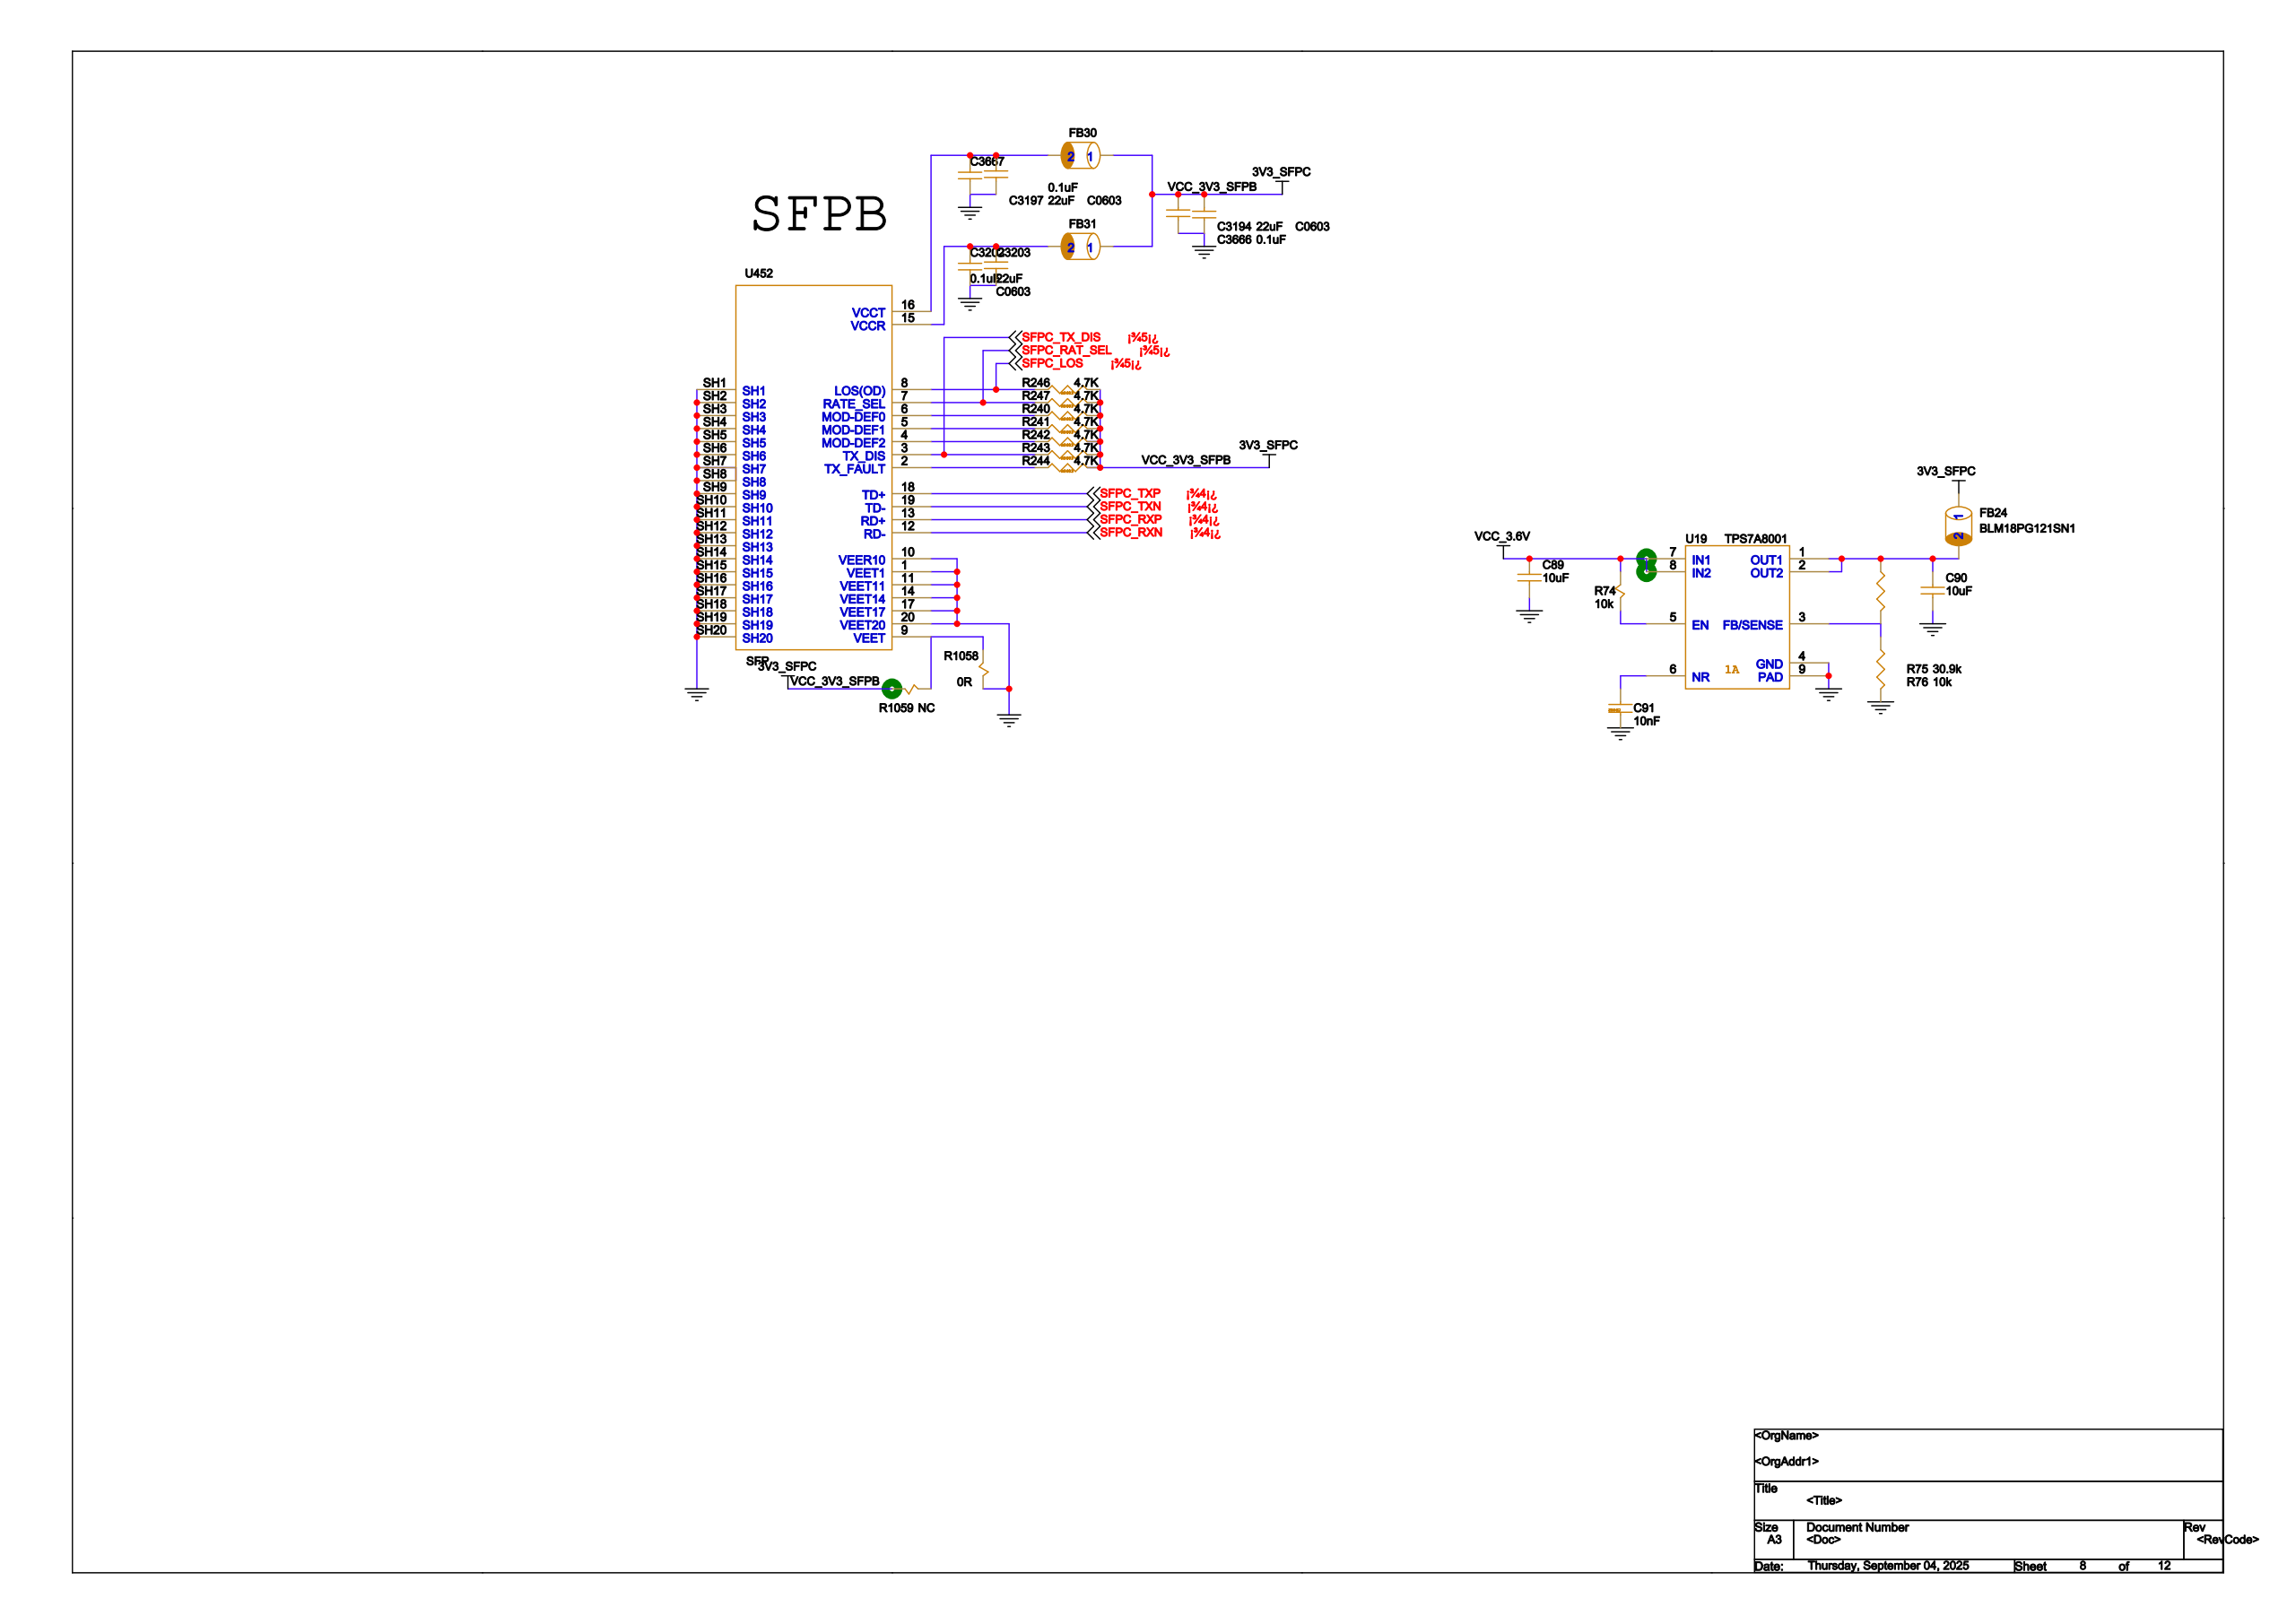Circuit board | Cadence Allegro | 528 parts | 530 nets | one sheet of the schematic
Parts on this sheet (reference | value | footprint):
C89 | 10uF | C0603
C90 | 10uF | C0603
C91 | 10nF | C0402
C3194 | 22uF | C0603
C3197 | 22uF | C0603
C3202 | 0.1uF | C0402
C3203 | 22uF | C0603
C3666 | 0.1uF | C0402
C3667 | 0.1uF | C0402
FB24 | BLM18PG121SN1 | 0603
FB30 | BLM18PG121SN1 | FB0603
FB31 | BLM18PG121SN1 | FB0603
R74 | 10k | R0402
R75 | 30.9k | R0402
R76 | 10k | R0402
R240 | 4.7K | R0402
R241 | 4.7K | R0402
R242 | 4.7K | R0402
R243 | 4.7K | R0402
R244 | 4.7K | R0402
R246 | 4.7K | R0402
R247 | 4.7K | R0402
R1058 | 0R | R0402
R1059 | NC | R0402
U19 | TPS7A8001 | TPS7A8001
U452 | SFP | MOL_74441-0001_CAGE_PFIT
Nets of these parts (net: part-pin ...):
GND: C89-2 C90-2 C91-1 C3194-2 C3197-2 C3202-1 C3203-2 C3666-1 C3667-1 R76-2 R1058-2 U19-4 U19-9 U452-1 U452-10 U452-11 U452-14 U452-17 U452-20 U452-SH1 U452-SH2 U452-SH3 U452-SH4 U452-SH5 U452-SH6 U452-SH7 U452-SH8 U452-SH9 U452-SH10 U452-SH11 U452-SH12 U452-SH13 U452-SH14 U452-SH15 U452-SH16 U452-SH17 U452-SH18 U452-SH19 U452-SH20
N18594995: R74-1 U19-5
N18595001: R75-2 R76-1 U19-3
VCC_3.6V: C89-1 R74-2 U19-7 U19-8
N18595017: C91-2 U19-6
N18594946: C90-1 FB24-2 R75-1 U19-1 U19-2
3V3_SFPC: C3194-1 C3666-2 FB24-1 FB30-1 FB31-1 R240-2 R241-2 R242-2 R243-2 R244-2 R246-2 R247-2 R1059-2
N18810814: C3197-1 C3667-2 FB30-2 U452-16
N18810887: C3202-2 C3203-1 FB31-2 U452-15
N18811190: R1058-1 R1059-1 U452-9
N18811039: R240-1 U452-6
N18811053: R241-1 U452-5
N18811067: R242-1 U452-4
SFPC_TX_DIS: R243-1 U452-3
N18811103: R244-1 U452-2
SFPC_LOS: R246-1 U452-8
SFPC_RAT_SEL: R247-1 U452-7
SFPC_TXP: U452-18
SFPC_TXN: U452-19
SFPC_RXP: U452-13
SFPC_RXN: U452-12